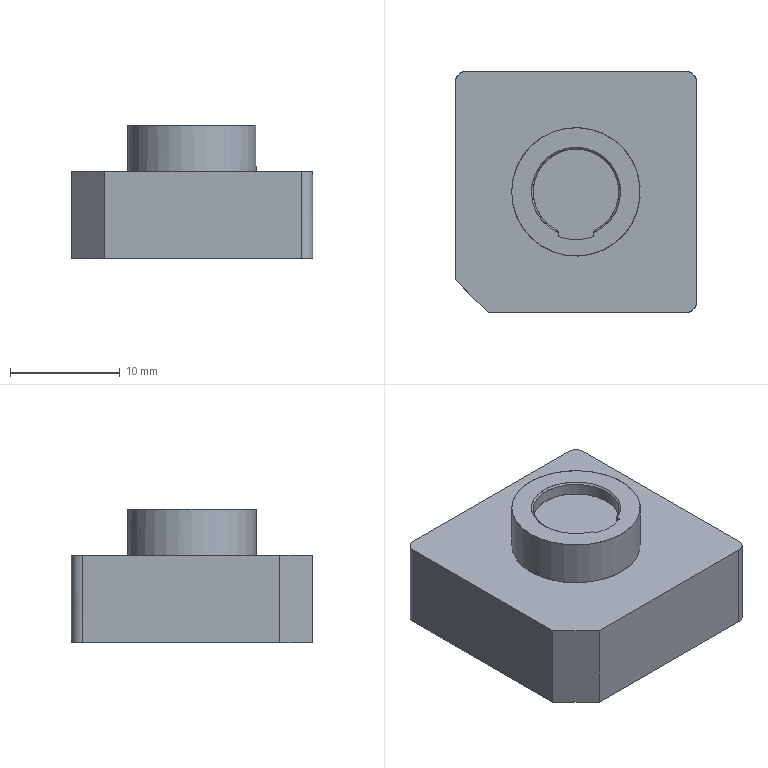NC program | PowerMill | posted by the shop | part box 22 x 22 x 12.219 mm
Lines 4804 to 5489 of 55612:
( TOOL ID   D10_1_1 )
( TOOL DIA. 10. TIP RAD 0 LENGTH 67.36 )
( Z = -.271 )
T3 M6
T12
G91 G28 Z0
G0 G90 G54
M08
S8500 M3
X0 Y0 M8
G43 Z11.799 H3
X16.607 Y.377
Z.929
G1 Z-.271 F360
X11.333 Y.253 F600
X-3.416 Y10.81
X-3.829 Y10.671
X-4.213 Y10.525
X-4.467 Y10.42
X-4.88 Y10.232
X-5.105 Y10.123
X-5.406 Y9.965
X-5.743 Y9.775
X-6.082 Y9.568
X-6.381 Y9.371
X-6.795 Y9.074
X-7.019 Y8.903
X-7.375 Y8.611
X-7.713 Y8.309
X10.351 Y-4.621
X10.202 Y-4.944
X10.123 Y-5.105
X9.965 Y-5.406
X9.775 Y-5.743
X9.58 Y-6.062
X9.371 Y-6.381
X9.072 Y-6.799
X8.93 Y-6.985
X8.642 Y-7.337
X8.361 Y-7.656
X8.082 Y-7.949
X7.713 Y-8.309
X-10.351 Y4.621
X-10.421 Y4.464
X-10.551 Y4.148
X-10.67 Y3.829
X-10.781 Y3.507
X-10.879 Y3.188
X-10.978 Y2.83
X-11.046 Y2.55
X-11.115 Y2.231
X-11.175 Y1.912
X-11.225 Y1.593
X-11.265 Y1.274
X-11.297 Y.955
X-11.319 Y.637
X-11.333 Y.318
X-11.336 Y-.126
X-11.333 Y-.253
X3.416 Y-10.81
G0 Z11.799
X0 Y0
Z9.799
X-21.393 Y-10.76
Z-3.22
G1 Z-4.42 F360
X-16.305 Y-9.369 F600
X-5.449 Y-9.827
X-5.834 Y-9.604
X-6.215 Y-9.362
X-6.675 Y-9.039
X-7.062 Y-8.741
X-7.38 Y-8.474
X-7.645 Y-8.236
X-7.982 Y-7.909
G2 X-8.505 Y-7.344 I8.827 J8.696
G1 X-8.741 Y-7.062
X-9.039 Y-6.675
X-9.362 Y-6.215
X-9.541 Y-5.934
X-9.714 Y-5.65
X-9.874 Y-5.364
X-10.026 Y-5.074
X-10.169 Y-4.781
X-10.288 Y-4.52
X-10.518 Y-3.955
X-10.734 Y-3.324
X-10.876 Y-2.825
X-11.008 Y-2.26
X-11.109 Y-1.695
X-11.18 Y-1.13
X-11.223 Y-.565
X-11.237 Y0
X-11.223 Y.565
X-11.18 Y1.13
X-11.109 Y1.695
X-11.008 Y2.26
X-10.876 Y2.825
X-10.714 Y3.39
X-10.518 Y3.955
X-10.288 Y4.52
X-10.169 Y4.781
G2 X-9.604 Y5.834 I10.387 J-4.898
G1 X-9.362 Y6.215
X-9.039 Y6.675
X-8.741 Y7.062
X-8.474 Y7.38
X-8.238 Y7.643
X-7.982 Y7.909
G2 X-7.344 Y8.505 I8.766 J-8.744
G1 X-7.062 Y8.741
X-6.675 Y9.039
X-6.215 Y9.362
X-5.834 Y9.604
G2 X-5.085 Y10.021 I6.078 J-10.039
G1 X-4.781 Y10.169
X-4.52 Y10.288
X-3.955 Y10.518
X-3.324 Y10.734
X-2.825 Y10.876
X-2.26 Y11.008
X-1.695 Y11.109
X-1.13 Y11.18
X-.565 Y11.223
X0 Y11.237
X.565 Y11.223
X1.13 Y11.18
X1.695 Y11.109
X2.26 Y11.008
X2.825 Y10.876
X3.39 Y10.714
X3.955 Y10.518
X4.52 Y10.288
X4.781 Y10.169
G2 X5.834 Y9.604 I-4.876 J-10.346
G1 X6.215 Y9.362
X6.675 Y9.039
X7.062 Y8.741
X7.38 Y8.474
X7.643 Y8.238
X7.982 Y7.909
X8.238 Y7.643
X8.551 Y7.291
X8.741 Y7.062
X8.954 Y6.79
X9.055 Y6.654
X9.362 Y6.215
X9.604 Y5.834
X9.714 Y5.65
X9.873 Y5.367
G2 X10.288 Y4.52 I-10.274 J-5.561
G1 X10.518 Y3.955
X10.734 Y3.324
X10.876 Y2.825
X11.008 Y2.26
X11.109 Y1.695
X11.18 Y1.13
X11.223 Y.565
X11.237 Y0
X11.223 Y-.565
X11.18 Y-1.13
X11.109 Y-1.695
X11.008 Y-2.26
X10.876 Y-2.825
X10.714 Y-3.39
X10.518 Y-3.955
X10.288 Y-4.52
X10.169 Y-4.781
G2 X9.604 Y-5.834 I-10.364 J4.886
G1 X9.362 Y-6.215
X9.039 Y-6.675
G2 X8.474 Y-7.38 I-9.879 J7.346
G1 X8.238 Y-7.643
X7.982 Y-7.909
G2 X7.344 Y-8.505 I-8.722 J8.697
X6.779 Y-8.962 I-8.259 J9.636
G1 X6.675 Y-9.039
X6.215 Y-9.362
X5.834 Y-9.604
G2 X4.772 Y-10.173 I-5.899 J9.728
G1 X4.52 Y-10.288
X3.955 Y-10.518
X3.324 Y-10.734
X2.825 Y-10.876
X2.26 Y-11.008
X1.695 Y-11.109
X1.13 Y-11.18
X.565 Y-11.223
X0 Y-11.237
X-.565 Y-11.223
X-1.13 Y-11.18
X-1.695 Y-11.109
X-2.26 Y-11.008
X-2.825 Y-10.876
X-3.39 Y-10.714
X-3.955 Y-10.518
X-4.52 Y-10.288
G2 X-5.449 Y-9.827 I4.603 J10.448
G0 Z9.799
Z10.799
X0 Y0
X8.745 Y-7.246
Z-3.19
G1 Z-4.39 F360
G3 X7.685 Y-7.685 I0 J-1.5 F600
G2 X-4.468 Y-9.905 I-7.683 J7.685
X4.988 Y9.655 I4.466 J9.906
X7.685 Y-7.685 I-4.986 J-9.655
G3 X7.245 Y-8.746 I1.061 J-1.061
G1 X8.689 Y-7.19
G3 X7.628 Y-7.629 I0 J-1.5
G2 X-4.435 Y-9.832 I-7.626 J7.629
X4.95 Y9.584 I4.433 J9.833
X7.628 Y-7.629 I-4.948 J-9.585
G3 X7.188 Y-8.69 I1.06 J-1.061
G0 Z10.799
X0 Y0
Z9.799
X16.34 Y-19.082
Z-11.12
G1 Z-12.32 F360
G3 X13.479 Y-14.982 I-1.43 J2.05 F600
G1 X13.324 Y-15.09
X13.322 Y-15.092
X13.32 Y-15.093
X13.004 Y-15.286
X13.002 Y-15.287
X12.999 Y-15.289
X12.683 Y-15.456
X12.681 Y-15.457
X12.679 Y-15.458
X12.363 Y-15.602
X12.361 Y-15.603
X12.359 Y-15.604
X12.042 Y-15.727
X12.04
X12.038 Y-15.728
X11.722 Y-15.831
X11.72 Y-15.832
X11.719
X11.53 Y-15.884
X11.529 Y-15.885
X11.528
X11.401 Y-15.916
X11.399 Y-15.917
X11.397
X11.081 Y-15.982
X11.079 Y-15.983
X11.077
X10.761 Y-16.032
X10.759
X10.757 Y-16.033
X10.441 Y-16.063
X10.439 Y-16.064
X10.437
X10.12 Y-16.079
X10.119
X10.117
X9.801 Y-16.08
X-7.904
X-7.905
X-8.221 Y-16.075
X-8.223
X-8.226
X-8.542 Y-16.051
X-8.545
X-8.547 Y-16.05
X-8.863 Y-16.006
X-8.866
X-8.868 Y-16.005
X-9.184 Y-15.94
X-9.187 Y-15.939
X-9.189
X-9.506 Y-15.852
X-9.508 Y-15.851
X-9.511 Y-15.85
X-9.827 Y-15.74
X-9.829 Y-15.739
X-9.832 Y-15.738
X-10.148 Y-15.603
X-10.151 Y-15.602
X-10.153 Y-15.601
X-10.469 Y-15.439
X-10.472 Y-15.438
X-10.474 Y-15.437
X-10.79 Y-15.245
X-10.793 Y-15.243
X-10.795 Y-15.242
X-11.112 Y-15.015
X-11.113 Y-15.014
X-11.115 Y-15.013
X-11.229 Y-14.921
X-11.231 Y-14.92
X-11.232 Y-14.919
X-11.434 Y-14.744
X-11.435 Y-14.742
X-11.437 Y-14.741
X-11.584 Y-14.601
Y-14.6
X-11.585 Y-14.599
X-14.599 Y-11.585
X-14.6 Y-11.584
X-14.601
X-14.741 Y-11.437
X-14.742 Y-11.435
X-14.744 Y-11.434
X-14.919 Y-11.232
X-14.92 Y-11.231
X-14.921 Y-11.229
X-15.013 Y-11.115
X-15.014 Y-11.113
X-15.015 Y-11.112
X-15.24 Y-10.798
X-15.242 Y-10.795
X-15.243 Y-10.793
X-15.437 Y-10.474
X-15.438 Y-10.472
X-15.439 Y-10.469
X-15.601 Y-10.153
X-15.602 Y-10.151
X-15.603 Y-10.148
X-15.738 Y-9.832
X-15.739 Y-9.829
X-15.74 Y-9.827
X-15.85 Y-9.511
X-15.851 Y-9.508
X-15.852 Y-9.506
X-15.939 Y-9.189
Y-9.187
X-15.94 Y-9.184
X-16.005 Y-8.868
X-16.006 Y-8.866
Y-8.863
X-16.05 Y-8.547
X-16.051 Y-8.545
Y-8.542
X-16.075 Y-8.226
Y-8.223
Y-8.221
X-16.08 Y-7.905
Y-7.904
Y9.801
X-16.079 Y10.117
Y10.119
Y10.12
X-16.064 Y10.436
Y10.439
Y10.441
X-16.033 Y10.757
X-16.032 Y10.759
Y10.761
X-15.984 Y11.077
X-15.983 Y11.079
Y11.081
X-15.917 Y11.398
Y11.4
X-15.916 Y11.402
X-15.832 Y11.718
Y11.72
X-15.831 Y11.722
X-15.728 Y12.038
X-15.727 Y12.04
X-15.726 Y12.042
X-15.604 Y12.359
X-15.603 Y12.361
X-15.602 Y12.363
X-15.458 Y12.679
X-15.457 Y12.681
X-15.456 Y12.683
X-15.289 Y12.999
X-15.287 Y13.001
X-15.286 Y13.004
X-15.094 Y13.32
X-15.092 Y13.322
X-15.091 Y13.324
X-14.87 Y13.64
X-14.868 Y13.642
X-14.867 Y13.644
X-14.613 Y13.96
X-14.611 Y13.963
X-14.609 Y13.965
X-14.317 Y14.281
X-14.315 Y14.283
X-14.313 Y14.285
X-13.974 Y14.601
X-13.972 Y14.603
X-13.969 Y14.605
X-13.644 Y14.867
X-13.642 Y14.868
X-13.64 Y14.87
X-13.324 Y15.09
X-13.322 Y15.092
X-13.32 Y15.093
X-13.004 Y15.286
X-13.002 Y15.287
X-12.999 Y15.289
X-12.683 Y15.456
X-12.681 Y15.457
X-12.679 Y15.458
X-12.363 Y15.602
X-12.361 Y15.603
X-12.359 Y15.604
X-12.042 Y15.727
X-12.04
X-12.038 Y15.728
X-11.722 Y15.831
X-11.72 Y15.832
X-11.718
X-11.402 Y15.916
X-11.4 Y15.917
X-11.397
X-11.081 Y15.982
X-11.079 Y15.983
X-11.077
X-10.761 Y16.032
X-10.759
X-10.757 Y16.033
X-10.441 Y16.063
X-10.439 Y16.064
X-10.437
X-10.12 Y16.079
X-10.119
X-10.117
X-9.801 Y16.08
X0
X9.801
X10.117 Y16.079
X10.119
X10.12
X10.436 Y16.064
X10.439
X10.441
X10.757 Y16.033
X10.759 Y16.032
X10.761
X11.077 Y15.984
X11.079 Y15.983
X11.081
X11.398 Y15.917
X11.4
X11.402 Y15.916
X11.718 Y15.832
X11.72
X11.722 Y15.831
X12.038 Y15.728
X12.04 Y15.727
X12.042 Y15.726
X12.359 Y15.604
X12.361 Y15.603
X12.363 Y15.602
X12.679 Y15.458
X12.681 Y15.457
X12.683 Y15.456
X12.999 Y15.289
X13.001 Y15.287
X13.004 Y15.286
X13.32 Y15.094
X13.322 Y15.092
X13.324 Y15.091
X13.64 Y14.87
X13.642 Y14.868
X13.644 Y14.867
X13.96 Y14.613
X13.963 Y14.611
X13.965 Y14.609
X14.281 Y14.317
X14.283 Y14.315
X14.285 Y14.313
X14.601 Y13.974
X14.603 Y13.972
X14.605 Y13.969
X14.867 Y13.644
X14.868 Y13.642
X14.87 Y13.64
X15.09 Y13.324
X15.092 Y13.322
X15.093 Y13.32
X15.286 Y13.004
X15.287 Y13.002
X15.289 Y12.999
X15.456 Y12.683
X15.457 Y12.681
X15.458 Y12.679
X15.602 Y12.363
X15.603 Y12.361
X15.604 Y12.359
X15.727 Y12.042
Y12.04
X15.728 Y12.038
X15.831 Y11.722
X15.832 Y11.72
Y11.718
X15.916 Y11.402
X15.917 Y11.4
Y11.397
X15.982 Y11.081
X15.983 Y11.079
Y11.077
X16.032 Y10.761
Y10.759
X16.033 Y10.757
X16.063 Y10.441
X16.064 Y10.439
Y10.437
X16.079 Y10.12
Y10.119
Y10.117
X16.08 Y9.801
Y-9.801
X16.079 Y-10.117
Y-10.119
Y-10.12
X16.064 Y-10.436
Y-10.439
Y-10.441
X16.033 Y-10.757
X16.032 Y-10.759
Y-10.761
X15.984 Y-11.077
X15.983 Y-11.079
Y-11.081
X15.917 Y-11.398
Y-11.4
X15.916 Y-11.402
X15.832 Y-11.718
Y-11.72
X15.831 Y-11.722
X15.728 Y-12.038
X15.727 Y-12.04
X15.726 Y-12.042
X15.604 Y-12.359
X15.603 Y-12.361
X15.602 Y-12.363
X15.458 Y-12.679
X15.457 Y-12.681
X15.456 Y-12.683
X15.289 Y-12.999
X15.287 Y-13.001
X15.286 Y-13.004
X15.094 Y-13.32
X15.092 Y-13.322
X15.091 Y-13.324
X14.87 Y-13.64
X14.868 Y-13.642
X14.867 Y-13.644
X14.613 Y-13.96
X14.611 Y-13.963
X14.609 Y-13.965
X14.317 Y-14.281
X14.315 Y-14.283
X14.313 Y-14.285
X13.974 Y-14.601
X13.972 Y-14.603
X13.969 Y-14.605
X13.644 Y-14.867
X13.642 Y-14.868
X13.64 Y-14.87
X13.479 Y-14.982
G3 X16.34 Y-19.082 I1.43 J-2.05
G1 X16.289 Y-19.021
G3 X13.428 Y-14.92 I-1.43 J2.05
G1 X13.278 Y-15.025
X12.962 Y-15.218
X12.646 Y-15.385
X12.33 Y-15.529
X12.014 Y-15.652
X11.697 Y-15.755
X11.508 Y-15.807
X11.381 Y-15.839
X11.065 Y-15.904
X10.749 Y-15.953
X10.433 Y-15.984
X10.117 Y-15.999
X9.801 Y-16.
X-7.904
X-8.22 Y-15.995
X-8.536 Y-15.971
X-8.852 Y-15.927
X-9.168 Y-15.862
X-9.484 Y-15.775
X-9.801 Y-15.665
X-10.117 Y-15.53
X-10.433 Y-15.368
X-10.749 Y-15.177
X-11.065 Y-14.95
X-11.18 Y-14.859
X-11.381 Y-14.683
X-11.528 Y-14.543
X-14.543 Y-11.528
X-14.683 Y-11.381
X-14.859 Y-11.18
X-14.95 Y-11.065
X-15.175 Y-10.751
X-15.368 Y-10.433
X-15.53 Y-10.117
X-15.665 Y-9.801
X-15.775 Y-9.484
X-15.862 Y-9.168
X-15.927 Y-8.852
X-15.971 Y-8.536
X-15.995 Y-8.22
X-16. Y-7.904
Y9.801
X-15.999 Y10.117
X-15.984 Y10.433
X-15.953 Y10.749
X-15.905 Y11.065
X-15.839 Y11.381
X-15.755 Y11.697
X-15.652 Y12.014
X-15.529 Y12.33
X-15.385 Y12.646
X-15.218 Y12.962
X-15.025 Y13.278
X-14.804 Y13.594
X-14.551 Y13.91
X-14.259 Y14.227
X-13.919 Y14.543
X-13.594 Y14.804
X-13.278 Y15.025
X-12.962 Y15.218
X-12.646 Y15.385
X-12.33 Y15.529
X-12.014 Y15.652
X-11.697 Y15.755
X-11.381 Y15.839
X-11.065 Y15.904
X-10.749 Y15.953
X-10.433 Y15.984
X-10.117 Y15.999
X-9.801 Y16.
X0
X9.801
X10.117 Y15.999
X10.433 Y15.984
X10.749 Y15.953
X11.065 Y15.905
X11.381 Y15.839
X11.697 Y15.755
X12.014 Y15.652
X12.33 Y15.529
X12.646 Y15.385
X12.962 Y15.218
X13.278 Y15.025
X13.594 Y14.804
X13.91 Y14.551
X14.227 Y14.259
X14.543 Y13.919
X14.804 Y13.594
X15.025 Y13.278
X15.218 Y12.962
X15.385 Y12.646
X15.529 Y12.33
X15.652 Y12.014
X15.755 Y11.697
X15.839 Y11.381
X15.904 Y11.065
X15.953 Y10.749
X15.984 Y10.433
X15.999 Y10.117
X16. Y9.801
Y-9.801
X15.999 Y-10.117
X15.984 Y-10.433
X15.953 Y-10.749
X15.905 Y-11.065
X15.839 Y-11.381
X15.755 Y-11.697
X15.652 Y-12.014
X15.529 Y-12.33
X15.385 Y-12.646
X15.218 Y-12.962
X15.025 Y-13.278
X14.804 Y-13.594
X14.551 Y-13.91
X14.259 Y-14.227
X13.919 Y-14.543
X13.594 Y-14.804
X13.428 Y-14.92
G3 X16.289 Y-19.021 I1.43 J-2.05
G0 Z9.799
Z10.799
X0 Y0
M9
M5
M01